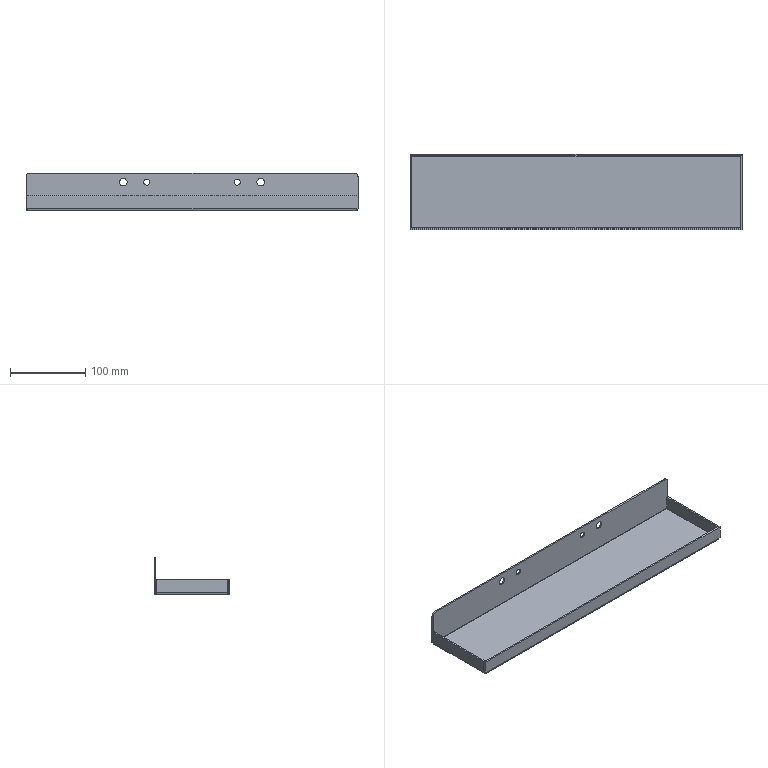Part | SolidWorks | features ICE 4, Extrusion 1, Fillet 1, FlatPattern 1, Rip 1, SheetMetal 1, Shell 1, SolidToSheetMetal 1 | 1 solid | 52 faces | box 440 x 100 x 50 mm | volume 150958 mm3 | plane 34 | cylinder 18 | commonest cylinder face diameters 10 x6 1 x4 5 x4 8 x4
STEP:
#1=CARTESIAN_POINT('',(-91.,50.,33.));
#2=VERTEX_POINT('',#1);
#3=CARTESIAN_POINT('',(-91.,50.,43.));
#4=VERTEX_POINT('',#3);
#5=CARTESIAN_POINT('',(-91.,50.,38.));
#6=DIRECTION('',(0.,1.,0.));
#7=DIRECTION('',(0.,0.,1.));
#8=AXIS2_PLACEMENT_3D('',#5,#6,#7);
#9=CIRCLE('',#8,5.);
#10=EDGE_CURVE('',#2,#4,#9,.T.);
#11=ORIENTED_EDGE('',*,*,#10,.T.);
#12=CARTESIAN_POINT('',(-91.,48.,43.));
#13=VERTEX_POINT('',#12);
#14=CARTESIAN_POINT('',(-91.,50.,43.));
#15=DIRECTION('',(0.,-1.,0.));
#16=VECTOR('',#15,1000.);
#17=LINE('',#14,#16);
#18=EDGE_CURVE('',#4,#13,#17,.T.);
#19=ORIENTED_EDGE('',*,*,#18,.T.);
#20=CARTESIAN_POINT('',(-91.,48.,33.));
#21=VERTEX_POINT('',#20);
#22=CARTESIAN_POINT('',(-91.,48.,38.));
#23=DIRECTION('',(0.,1.,0.));
#24=DIRECTION('',(0.,0.,1.));
#25=AXIS2_PLACEMENT_3D('',#22,#23,#24);
#26=CIRCLE('',#25,5.);
#27=EDGE_CURVE('',#21,#13,#26,.T.);
#28=ORIENTED_EDGE('',*,*,#27,.F.);
#29=CARTESIAN_POINT('',(-91.,50.,33.));
#30=DIRECTION('',(0.,-1.,0.));
#31=VECTOR('',#30,1000.);
#32=LINE('',#29,#31);
#33=EDGE_CURVE('',#2,#21,#32,.T.);
#34=ORIENTED_EDGE('',*,*,#33,.F.);
#35=EDGE_LOOP('',(#11,#19,#28,#34));
#36=FACE_OUTER_BOUND('',#35,.T.);
#37=CARTESIAN_POINT('',(-91.,50.,38.));
#38=DIRECTION('',(0.,-1.,0.));
#39=DIRECTION('',(0.,0.,-1.));
#40=AXIS2_PLACEMENT_3D('',#37,#38,#39);
#41=CYLINDRICAL_SURFACE('',#40,5.);
#42=ADVANCED_FACE('',(#36),#41,.F.);
#43=CARTESIAN_POINT('',(91.,50.,33.));
#44=VERTEX_POINT('',#43);
#45=CARTESIAN_POINT('',(91.,50.,43.));
#46=VERTEX_POINT('',#45);
#47=CARTESIAN_POINT('',(91.,50.,38.));
#48=DIRECTION('',(0.,1.,0.));
#49=DIRECTION('',(0.,0.,1.));
#50=AXIS2_PLACEMENT_3D('',#47,#48,#49);
#51=CIRCLE('',#50,5.);
#52=EDGE_CURVE('',#44,#46,#51,.T.);
#53=ORIENTED_EDGE('',*,*,#52,.T.);
#54=CARTESIAN_POINT('',(91.,48.,43.));
#55=VERTEX_POINT('',#54);
#56=CARTESIAN_POINT('',(91.,50.,43.));
#57=DIRECTION('',(0.,-1.,0.));
#58=VECTOR('',#57,1000.);
#59=LINE('',#56,#58);
#60=EDGE_CURVE('',#46,#55,#59,.T.);
#61=ORIENTED_EDGE('',*,*,#60,.T.);
#62=CARTESIAN_POINT('',(91.,48.,33.));
#63=VERTEX_POINT('',#62);
#64=CARTESIAN_POINT('',(91.,48.,38.));
#65=DIRECTION('',(0.,1.,0.));
#66=DIRECTION('',(0.,0.,1.));
#67=AXIS2_PLACEMENT_3D('',#64,#65,#66);
#68=CIRCLE('',#67,5.);
#69=EDGE_CURVE('',#63,#55,#68,.T.);
#70=ORIENTED_EDGE('',*,*,#69,.F.);
#71=CARTESIAN_POINT('',(91.,50.,33.));
#72=DIRECTION('',(0.,-1.,0.));
#73=VECTOR('',#72,1000.);
#74=LINE('',#71,#73);
#75=EDGE_CURVE('',#44,#63,#74,.T.);
#76=ORIENTED_EDGE('',*,*,#75,.F.);
#77=EDGE_LOOP('',(#53,#61,#70,#76));
#78=FACE_OUTER_BOUND('',#77,.T.);
#79=CARTESIAN_POINT('',(91.,50.,38.));
#80=DIRECTION('',(0.,-1.,0.));
#81=DIRECTION('',(0.,0.,-1.));
#82=AXIS2_PLACEMENT_3D('',#79,#80,#81);
#83=CYLINDRICAL_SURFACE('',#82,5.);
#84=ADVANCED_FACE('',(#78),#83,.F.);
#85=CARTESIAN_POINT('',(60.,50.,42.));
#86=VERTEX_POINT('',#85);
#87=CARTESIAN_POINT('',(60.,50.,34.));
#88=VERTEX_POINT('',#87);
#89=CARTESIAN_POINT('',(60.,50.,38.));
#90=DIRECTION('',(0.,-1.,0.));
#91=DIRECTION('',(0.,0.,-1.));
#92=AXIS2_PLACEMENT_3D('',#89,#90,#91);
#93=CIRCLE('',#92,4.);
#94=EDGE_CURVE('',#86,#88,#93,.T.);
#95=ORIENTED_EDGE('',*,*,#94,.F.);
#96=CARTESIAN_POINT('',(60.,48.,42.));
#97=VERTEX_POINT('',#96);
#98=CARTESIAN_POINT('',(60.,50.,42.));
#99=DIRECTION('',(0.,-1.,0.));
#100=VECTOR('',#99,1000.);
#101=LINE('',#98,#100);
#102=EDGE_CURVE('',#86,#97,#101,.T.);
#103=ORIENTED_EDGE('',*,*,#102,.T.);
#104=CARTESIAN_POINT('',(60.,48.,34.));
#105=VERTEX_POINT('',#104);
#106=CARTESIAN_POINT('',(60.,48.,38.));
#107=DIRECTION('',(0.,-1.,0.));
#108=DIRECTION('',(0.,0.,-1.));
#109=AXIS2_PLACEMENT_3D('',#106,#107,#108);
#110=CIRCLE('',#109,4.);
#111=EDGE_CURVE('',#97,#105,#110,.T.);
#112=ORIENTED_EDGE('',*,*,#111,.T.);
#113=CARTESIAN_POINT('',(60.,50.,34.));
#114=DIRECTION('',(0.,-1.,0.));
#115=VECTOR('',#114,1000.);
#116=LINE('',#113,#115);
#117=EDGE_CURVE('',#88,#105,#116,.T.);
#118=ORIENTED_EDGE('',*,*,#117,.F.);
#119=EDGE_LOOP('',(#95,#103,#112,#118));
#120=FACE_OUTER_BOUND('',#119,.T.);
#121=CARTESIAN_POINT('',(60.,50.,38.));
#122=DIRECTION('',(0.,-1.,0.));
#123=DIRECTION('',(0.,0.,-1.));
#124=AXIS2_PLACEMENT_3D('',#121,#122,#123);
#125=CYLINDRICAL_SURFACE('',#124,4.);
#126=ADVANCED_FACE('',(#120),#125,.F.);
#127=CARTESIAN_POINT('',(-60.,50.,42.));
#128=VERTEX_POINT('',#127);
#129=CARTESIAN_POINT('',(-60.,50.,34.));
#130=VERTEX_POINT('',#129);
#131=CARTESIAN_POINT('',(-60.,50.,38.));
#132=DIRECTION('',(0.,-1.,0.));
#133=DIRECTION('',(0.,0.,-1.));
#134=AXIS2_PLACEMENT_3D('',#131,#132,#133);
#135=CIRCLE('',#134,4.);
#136=EDGE_CURVE('',#128,#130,#135,.T.);
#137=ORIENTED_EDGE('',*,*,#136,.F.);
#138=CARTESIAN_POINT('',(-60.,48.,42.));
#139=VERTEX_POINT('',#138);
#140=CARTESIAN_POINT('',(-60.,50.,42.));
#141=DIRECTION('',(0.,-1.,0.));
#142=VECTOR('',#141,1000.);
#143=LINE('',#140,#142);
#144=EDGE_CURVE('',#128,#139,#143,.T.);
#145=ORIENTED_EDGE('',*,*,#144,.T.);
#146=CARTESIAN_POINT('',(-60.,48.,34.));
#147=VERTEX_POINT('',#146);
#148=CARTESIAN_POINT('',(-60.,48.,38.));
#149=DIRECTION('',(0.,-1.,0.));
#150=DIRECTION('',(0.,0.,-1.));
#151=AXIS2_PLACEMENT_3D('',#148,#149,#150);
#152=CIRCLE('',#151,4.);
#153=EDGE_CURVE('',#139,#147,#152,.T.);
#154=ORIENTED_EDGE('',*,*,#153,.T.);
#155=CARTESIAN_POINT('',(-60.,50.,34.));
#156=DIRECTION('',(0.,-1.,0.));
#157=VECTOR('',#156,1000.);
#158=LINE('',#155,#157);
#159=EDGE_CURVE('',#130,#147,#158,.T.);
#160=ORIENTED_EDGE('',*,*,#159,.F.);
#161=EDGE_LOOP('',(#137,#145,#154,#160));
#162=FACE_OUTER_BOUND('',#161,.T.);
#163=CARTESIAN_POINT('',(-60.,50.,38.));
#164=DIRECTION('',(0.,-1.,0.));
#165=DIRECTION('',(0.,0.,-1.));
#166=AXIS2_PLACEMENT_3D('',#163,#164,#165);
#167=CYLINDRICAL_SURFACE('',#166,4.);
#168=ADVANCED_FACE('',(#162),#167,.F.);
#169=CARTESIAN_POINT('',(-217.5,47.5,2.));
#170=VERTEX_POINT('',#169);
#171=CARTESIAN_POINT('',(-217.5,47.5,0.));
#172=VERTEX_POINT('',#171);
#173=CARTESIAN_POINT('',(-217.5,47.5,0.));
#174=DIRECTION('',(0.,0.,-1.));
#175=VECTOR('',#174,1000.);
#176=LINE('',#173,#175);
#177=EDGE_CURVE('',#170,#172,#176,.T.);
#178=ORIENTED_EDGE('',*,*,#177,.F.);
#179=CARTESIAN_POINT('',(-217.5,48.,2.5));
#180=VERTEX_POINT('',#179);
#181=CARTESIAN_POINT('',(-217.5,47.5,2.5));
#182=DIRECTION('',(1.,0.,0.));
#183=DIRECTION('',(0.,0.,1.));
#184=AXIS2_PLACEMENT_3D('',#181,#182,#183);
#185=CIRCLE('',#184,0.5);
#186=EDGE_CURVE('',#170,#180,#185,.T.);
#187=ORIENTED_EDGE('',*,*,#186,.T.);
#188=CARTESIAN_POINT('',(-217.5,50.,2.5));
#189=VERTEX_POINT('',#188);
#190=CARTESIAN_POINT('',(-217.5,50.,2.5));
#191=DIRECTION('',(0.,1.,0.));
#192=VECTOR('',#191,1000.);
#193=LINE('',#190,#192);
#194=EDGE_CURVE('',#180,#189,#193,.T.);
#195=ORIENTED_EDGE('',*,*,#194,.T.);
#196=CARTESIAN_POINT('',(-217.5,47.5,2.5));
#197=DIRECTION('',(1.,0.,0.));
#198=DIRECTION('',(0.,0.,1.));
#199=AXIS2_PLACEMENT_3D('',#196,#197,#198);
#200=CIRCLE('',#199,2.5);
#201=EDGE_CURVE('',#172,#189,#200,.T.);
#202=ORIENTED_EDGE('',*,*,#201,.F.);
#203=EDGE_LOOP('',(#178,#187,#195,#202));
#204=FACE_OUTER_BOUND('',#203,.T.);
#205=CARTESIAN_POINT('',(-217.5,47.5,2.5));
#206=DIRECTION('',(1.,0.,0.));
#207=DIRECTION('',(0.,0.,-1.));
#208=AXIS2_PLACEMENT_3D('',#205,#206,#207);
#209=PLANE('',#208);
#210=ADVANCED_FACE('',(#204),#209,.F.);
#211=ORIENTED_EDGE('',*,*,#194,.F.);
#212=CARTESIAN_POINT('',(-220.,48.,2.5));
#213=VERTEX_POINT('',#212);
#214=CARTESIAN_POINT('',(-220.,48.,2.5));
#215=DIRECTION('',(1.,0.,0.));
#216=VECTOR('',#215,1000.);
#217=LINE('',#214,#216);
#218=EDGE_CURVE('',#213,#180,#217,.T.);
#219=ORIENTED_EDGE('',*,*,#218,.F.);
#220=CARTESIAN_POINT('',(-220.,50.,2.5));
#221=VERTEX_POINT('',#220);
#222=CARTESIAN_POINT('',(-220.,50.,2.5));
#223=DIRECTION('',(0.,1.,0.));
#224=VECTOR('',#223,1000.);
#225=LINE('',#222,#224);
#226=EDGE_CURVE('',#213,#221,#225,.T.);
#227=ORIENTED_EDGE('',*,*,#226,.T.);
#228=CARTESIAN_POINT('',(-220.,50.,2.5));
#229=DIRECTION('',(1.,0.,0.));
#230=VECTOR('',#229,1000.);
#231=LINE('',#228,#230);
#232=EDGE_CURVE('',#221,#189,#231,.T.);
#233=ORIENTED_EDGE('',*,*,#232,.T.);
#234=EDGE_LOOP('',(#211,#219,#227,#233));
#235=FACE_OUTER_BOUND('',#234,.T.);
#236=CARTESIAN_POINT('',(-220.,50.,2.5));
#237=DIRECTION('',(0.,0.,-1.));
#238=DIRECTION('',(1.,0.,0.));
#239=AXIS2_PLACEMENT_3D('',#236,#237,#238);
#240=PLANE('',#239);
#241=ADVANCED_FACE('',(#235),#240,.T.);
#242=ORIENTED_EDGE('',*,*,#226,.F.);
#243=CARTESIAN_POINT('',(-220.,48.,45.));
#244=VERTEX_POINT('',#243);
#245=CARTESIAN_POINT('',(-220.,48.,20.));
#246=DIRECTION('',(0.,0.,-1.));
#247=VECTOR('',#246,1000.);
#248=LINE('',#245,#247);
#249=EDGE_CURVE('',#244,#213,#248,.T.);
#250=ORIENTED_EDGE('',*,*,#249,.F.);
#251=CARTESIAN_POINT('',(-220.,50.,45.));
#252=VERTEX_POINT('',#251);
#253=CARTESIAN_POINT('',(-220.,50.,45.));
#254=DIRECTION('',(0.,1.,0.));
#255=VECTOR('',#254,1000.);
#256=LINE('',#253,#255);
#257=EDGE_CURVE('',#244,#252,#256,.T.);
#258=ORIENTED_EDGE('',*,*,#257,.T.);
#259=CARTESIAN_POINT('',(-220.,50.,20.));
#260=DIRECTION('',(0.,0.,-1.));
#261=VECTOR('',#260,1000.);
#262=LINE('',#259,#261);
#263=EDGE_CURVE('',#252,#221,#262,.T.);
#264=ORIENTED_EDGE('',*,*,#263,.T.);
#265=EDGE_LOOP('',(#242,#250,#258,#264));
#266=FACE_OUTER_BOUND('',#265,.T.);
#267=CARTESIAN_POINT('',(-220.,50.,20.));
#268=DIRECTION('',(-1.,0.,0.));
#269=DIRECTION('',(0.,0.,-1.));
#270=AXIS2_PLACEMENT_3D('',#267,#268,#269);
#271=PLANE('',#270);
#272=ADVANCED_FACE('',(#266),#271,.T.);
#273=ORIENTED_EDGE('',*,*,#257,.F.);
#274=CARTESIAN_POINT('',(-215.,48.,50.));
#275=VERTEX_POINT('',#274);
#276=CARTESIAN_POINT('',(-215.,48.,45.));
#277=DIRECTION('',(0.,1.,0.));
#278=DIRECTION('',(0.,0.,-1.));
#279=AXIS2_PLACEMENT_3D('',#276,#277,#278);
#280=CIRCLE('',#279,5.);
#281=EDGE_CURVE('',#244,#275,#280,.T.);
#282=ORIENTED_EDGE('',*,*,#281,.T.);
#283=CARTESIAN_POINT('',(-215.,50.,50.));
#284=VERTEX_POINT('',#283);
#285=CARTESIAN_POINT('',(-215.,50.,50.));
#286=DIRECTION('',(0.,1.,0.));
#287=VECTOR('',#286,1000.);
#288=LINE('',#285,#287);
#289=EDGE_CURVE('',#275,#284,#288,.T.);
#290=ORIENTED_EDGE('',*,*,#289,.T.);
#291=CARTESIAN_POINT('',(-215.,50.,45.));
#292=DIRECTION('',(0.,1.,0.));
#293=DIRECTION('',(0.,0.,-1.));
#294=AXIS2_PLACEMENT_3D('',#291,#292,#293);
#295=CIRCLE('',#294,5.);
#296=EDGE_CURVE('',#252,#284,#295,.T.);
#297=ORIENTED_EDGE('',*,*,#296,.F.);
#298=EDGE_LOOP('',(#273,#282,#290,#297));
#299=FACE_OUTER_BOUND('',#298,.T.);
#300=CARTESIAN_POINT('',(-215.,50.,45.));
#301=DIRECTION('',(0.,-1.,0.));
#302=DIRECTION('',(0.,0.,-1.));
#303=AXIS2_PLACEMENT_3D('',#300,#301,#302);
#304=CYLINDRICAL_SURFACE('',#303,5.);
#305=ADVANCED_FACE('',(#299),#304,.T.);
#306=ORIENTED_EDGE('',*,*,#289,.F.);
#307=CARTESIAN_POINT('',(215.,48.,50.));
#308=VERTEX_POINT('',#307);
#309=CARTESIAN_POINT('',(-220.,48.,50.));
#310=DIRECTION('',(1.,0.,0.));
#311=VECTOR('',#310,1000.);
#312=LINE('',#309,#311);
#313=EDGE_CURVE('',#275,#308,#312,.T.);
#314=ORIENTED_EDGE('',*,*,#313,.T.);
#315=CARTESIAN_POINT('',(215.,50.,50.));
#316=VERTEX_POINT('',#315);
#317=CARTESIAN_POINT('',(215.,50.,50.));
#318=DIRECTION('',(0.,1.,0.));
#319=VECTOR('',#318,1000.);
#320=LINE('',#317,#319);
#321=EDGE_CURVE('',#308,#316,#320,.T.);
#322=ORIENTED_EDGE('',*,*,#321,.T.);
#323=CARTESIAN_POINT('',(220.,50.,50.));
#324=DIRECTION('',(1.,0.,0.));
#325=VECTOR('',#324,1000.);
#326=LINE('',#323,#325);
#327=EDGE_CURVE('',#284,#316,#326,.T.);
#328=ORIENTED_EDGE('',*,*,#327,.F.);
#329=EDGE_LOOP('',(#306,#314,#322,#328));
#330=FACE_OUTER_BOUND('',#329,.T.);
#331=CARTESIAN_POINT('',(220.,50.,50.));
#332=DIRECTION('',(0.,0.,-1.));
#333=DIRECTION('',(1.,0.,0.));
#334=AXIS2_PLACEMENT_3D('',#331,#332,#333);
#335=PLANE('',#334);
#336=ADVANCED_FACE('',(#330),#335,.F.);
#337=ORIENTED_EDGE('',*,*,#321,.F.);
#338=CARTESIAN_POINT('',(220.,48.,45.));
#339=VERTEX_POINT('',#338);
#340=CARTESIAN_POINT('',(215.,48.,45.));
#341=DIRECTION('',(0.,1.,0.));
#342=DIRECTION('',(0.,0.,-1.));
#343=AXIS2_PLACEMENT_3D('',#340,#341,#342);
#344=CIRCLE('',#343,5.);
#345=EDGE_CURVE('',#308,#339,#344,.T.);
#346=ORIENTED_EDGE('',*,*,#345,.T.);
#347=CARTESIAN_POINT('',(220.,50.,45.));
#348=VERTEX_POINT('',#347);
#349=CARTESIAN_POINT('',(220.,50.,45.));
#350=DIRECTION('',(0.,1.,0.));
#351=VECTOR('',#350,1000.);
#352=LINE('',#349,#351);
#353=EDGE_CURVE('',#339,#348,#352,.T.);
#354=ORIENTED_EDGE('',*,*,#353,.T.);
#355=CARTESIAN_POINT('',(215.,50.,45.));
#356=DIRECTION('',(0.,1.,0.));
#357=DIRECTION('',(0.,0.,-1.));
#358=AXIS2_PLACEMENT_3D('',#355,#356,#357);
#359=CIRCLE('',#358,5.);
#360=EDGE_CURVE('',#316,#348,#359,.T.);
#361=ORIENTED_EDGE('',*,*,#360,.F.);
#362=EDGE_LOOP('',(#337,#346,#354,#361));
#363=FACE_OUTER_BOUND('',#362,.T.);
#364=CARTESIAN_POINT('',(215.,50.,45.));
#365=DIRECTION('',(0.,-1.,0.));
#366=DIRECTION('',(0.,0.,-1.));
#367=AXIS2_PLACEMENT_3D('',#364,#365,#366);
#368=CYLINDRICAL_SURFACE('',#367,5.);
#369=ADVANCED_FACE('',(#363),#368,.T.);
#370=ORIENTED_EDGE('',*,*,#353,.F.);
#371=CARTESIAN_POINT('',(220.,48.,2.5));
#372=VERTEX_POINT('',#371);
#373=CARTESIAN_POINT('',(220.,48.,20.));
#374=DIRECTION('',(0.,0.,-1.));
#375=VECTOR('',#374,1000.);
#376=LINE('',#373,#375);
#377=EDGE_CURVE('',#339,#372,#376,.T.);
#378=ORIENTED_EDGE('',*,*,#377,.T.);
#379=CARTESIAN_POINT('',(220.,50.,2.5));
#380=VERTEX_POINT('',#379);
#381=CARTESIAN_POINT('',(220.,50.,2.5));
#382=DIRECTION('',(0.,1.,0.));
#383=VECTOR('',#382,1000.);
#384=LINE('',#381,#383);
#385=EDGE_CURVE('',#372,#380,#384,.T.);
#386=ORIENTED_EDGE('',*,*,#385,.T.);
#387=CARTESIAN_POINT('',(220.,50.,20.));
#388=DIRECTION('',(0.,0.,-1.));
#389=VECTOR('',#388,1000.);
#390=LINE('',#387,#389);
#391=EDGE_CURVE('',#348,#380,#390,.T.);
#392=ORIENTED_EDGE('',*,*,#391,.F.);
#393=EDGE_LOOP('',(#370,#378,#386,#392));
#394=FACE_OUTER_BOUND('',#393,.T.);
#395=CARTESIAN_POINT('',(220.,50.,20.));
#396=DIRECTION('',(-1.,0.,0.));
#397=DIRECTION('',(0.,0.,-1.));
#398=AXIS2_PLACEMENT_3D('',#395,#396,#397);
#399=PLANE('',#398);
#400=ADVANCED_FACE('',(#394),#399,.F.);
#401=ORIENTED_EDGE('',*,*,#385,.F.);
#402=CARTESIAN_POINT('',(217.5,48.,2.5));
#403=VERTEX_POINT('',#402);
#404=CARTESIAN_POINT('',(-220.,48.,2.5));
#405=DIRECTION('',(1.,0.,0.));
#406=VECTOR('',#405,1000.);
#407=LINE('',#404,#406);
#408=EDGE_CURVE('',#403,#372,#407,.T.);
#409=ORIENTED_EDGE('',*,*,#408,.F.);
#410=CARTESIAN_POINT('',(217.5,50.,2.5));
#411=VERTEX_POINT('',#410);
#412=CARTESIAN_POINT('',(217.5,50.,2.5));
#413=DIRECTION('',(0.,1.,0.));
#414=VECTOR('',#413,1000.);
#415=LINE('',#412,#414);
#416=EDGE_CURVE('',#403,#411,#415,.T.);
#417=ORIENTED_EDGE('',*,*,#416,.T.);
#418=CARTESIAN_POINT('',(220.,50.,2.5));
#419=DIRECTION('',(1.,0.,0.));
#420=VECTOR('',#419,1000.);
#421=LINE('',#418,#420);
#422=EDGE_CURVE('',#411,#380,#421,.T.);
#423=ORIENTED_EDGE('',*,*,#422,.T.);
#424=EDGE_LOOP('',(#401,#409,#417,#423));
#425=FACE_OUTER_BOUND('',#424,.T.);
#426=CARTESIAN_POINT('',(220.,50.,2.5));
#427=DIRECTION('',(0.,0.,-1.));
#428=DIRECTION('',(1.,0.,0.));
#429=AXIS2_PLACEMENT_3D('',#426,#427,#428);
#430=PLANE('',#429);
#431=ADVANCED_FACE('',(#425),#430,.T.);
#432=ORIENTED_EDGE('',*,*,#416,.F.);
#433=CARTESIAN_POINT('',(217.5,47.5,2.));
#434=VERTEX_POINT('',#433);
#435=CARTESIAN_POINT('',(217.5,47.5,2.5));
#436=DIRECTION('',(-1.,0.,0.));
#437=DIRECTION('',(0.,0.,1.));
#438=AXIS2_PLACEMENT_3D('',#435,#436,#437);
#439=CIRCLE('',#438,0.5);
#440=EDGE_CURVE('',#403,#434,#439,.T.);
#441=ORIENTED_EDGE('',*,*,#440,.T.);
#442=CARTESIAN_POINT('',(217.5,47.5,0.));
#443=VERTEX_POINT('',#442);
#444=CARTESIAN_POINT('',(217.5,47.5,0.));
#445=DIRECTION('',(0.,0.,-1.));
#446=VECTOR('',#445,1000.);
#447=LINE('',#444,#446);
#448=EDGE_CURVE('',#434,#443,#447,.T.);
#449=ORIENTED_EDGE('',*,*,#448,.T.);
#450=CARTESIAN_POINT('',(217.5,47.5,2.5));
#451=DIRECTION('',(-1.,0.,0.));
#452=DIRECTION('',(0.,0.,1.));
#453=AXIS2_PLACEMENT_3D('',#450,#451,#452);
#454=CIRCLE('',#453,2.5);
#455=EDGE_CURVE('',#411,#443,#454,.T.);
#456=ORIENTED_EDGE('',*,*,#455,.F.);
#457=EDGE_LOOP('',(#432,#441,#449,#456));
#458=FACE_OUTER_BOUND('',#457,.T.);
#459=CARTESIAN_POINT('',(217.5,47.5,2.5));
#460=DIRECTION('',(1.,0.,0.));
#461=DIRECTION('',(0.,0.,-1.));
#462=AXIS2_PLACEMENT_3D('',#459,#460,#461);
#463=PLANE('',#462);
#464=ADVANCED_FACE('',(#458),#463,.T.);
#465=ORIENTED_EDGE('',*,*,#448,.F.);
#466=CARTESIAN_POINT('',(218.,47.5,2.5));
#467=VERTEX_POINT('',#466);
#468=CARTESIAN_POINT('',(217.5,47.5,2.5));
#469=DIRECTION('',(0.,-1.,0.));
#470=DIRECTION('',(-1.,0.,0.));
#471=AXIS2_PLACEMENT_3D('',#468,#469,#470);
#472=CIRCLE('',#471,0.5);
#473=EDGE_CURVE('',#434,#467,#472,.T.);
#474=ORIENTED_EDGE('',*,*,#473,.T.);
#475=CARTESIAN_POINT('',(220.,47.5,2.5));
#476=VERTEX_POINT('',#475);
#477=CARTESIAN_POINT('',(220.,47.5,2.5));
#478=DIRECTION('',(1.,0.,0.));
#479=VECTOR('',#478,1000.);
#480=LINE('',#477,#479);
#481=EDGE_CURVE('',#467,#476,#480,.T.);
#482=ORIENTED_EDGE('',*,*,#481,.T.);
#483=CARTESIAN_POINT('',(217.5,47.5,2.5));
#484=DIRECTION('',(0.,-1.,0.));
#485=DIRECTION('',(0.,0.,-1.));
#486=AXIS2_PLACEMENT_3D('',#483,#484,#485);
#487=CIRCLE('',#486,2.5);
#488=EDGE_CURVE('',#443,#476,#487,.T.);
#489=ORIENTED_EDGE('',*,*,#488,.F.);
#490=EDGE_LOOP('',(#465,#474,#482,#489));
#491=FACE_OUTER_BOUND('',#490,.T.);
#492=CARTESIAN_POINT('',(217.5,47.5,2.5));
#493=DIRECTION('',(0.,1.,0.));
#494=DIRECTION('',(0.,0.,1.));
#495=AXIS2_PLACEMENT_3D('',#492,#493,#494);
#496=PLANE('',#495);
#497=ADVANCED_FACE('',(#491),#496,.T.);
#498=ORIENTED_EDGE('',*,*,#481,.F.);
#499=CARTESIAN_POINT('',(218.,47.5,20.));
#500=VERTEX_POINT('',#499);
#501=CARTESIAN_POINT('',(218.,47.5,20.));
#502=DIRECTION('',(0.,0.,1.));
#503=VECTOR('',#502,1000.);
#504=LINE('',#501,#503);
#505=EDGE_CURVE('',#467,#500,#504,.T.);
#506=ORIENTED_EDGE('',*,*,#505,.T.);
#507=CARTESIAN_POINT('',(220.,47.5,20.));
#508=VERTEX_POINT('',#507);
#509=CARTESIAN_POINT('',(220.,47.5,20.));
#510=DIRECTION('',(1.,0.,0.));
#511=VECTOR('',#510,1000.);
#512=LINE('',#509,#511);
#513=EDGE_CURVE('',#500,#508,#512,.T.);
#514=ORIENTED_EDGE('',*,*,#513,.T.);
#515=CARTESIAN_POINT('',(220.,47.5,-11.));
#516=DIRECTION('',(0.,0.,1.));
#517=VECTOR('',#516,1000.);
#518=LINE('',#515,#517);
#519=EDGE_CURVE('',#476,#508,#518,.T.);
#520=ORIENTED_EDGE('',*,*,#519,.F.);
#521=EDGE_LOOP('',(#498,#506,#514,#520));
#522=FACE_OUTER_BOUND('',#521,.T.);
#523=CARTESIAN_POINT('',(220.,47.5,-11.));
#524=DIRECTION('',(0.,-1.,0.));
#525=DIRECTION('',(0.,0.,1.));
#526=AXIS2_PLACEMENT_3D('',#523,#524,#525);
#527=PLANE('',#526);
#528=ADVANCED_FACE('',(#522),#527,.F.);
#529=ORIENTED_EDGE('',*,*,#513,.F.);
#530=CARTESIAN_POINT('',(218.,-47.5,20.));
#531=VERTEX_POINT('',#530);
#532=CARTESIAN_POINT('',(218.,50.,20.));
#533=DIRECTION('',(0.,1.,0.));
#534=VECTOR('',#533,1000.);
#535=LINE('',#532,#534);
#536=EDGE_CURVE('',#531,#500,#535,.T.);
#537=ORIENTED_EDGE('',*,*,#536,.F.);
#538=CARTESIAN_POINT('',(220.,-47.5,20.));
#539=VERTEX_POINT('',#538);
#540=CARTESIAN_POINT('',(220.,-47.5,20.));
#541=DIRECTION('',(1.,0.,0.));
#542=VECTOR('',#541,1000.);
#543=LINE('',#540,#542);
#544=EDGE_CURVE('',#531,#539,#543,.T.);
#545=ORIENTED_EDGE('',*,*,#544,.T.);
#546=CARTESIAN_POINT('',(220.,50.,20.));
#547=DIRECTION('',(0.,1.,0.));
#548=VECTOR('',#547,1000.);
#549=LINE('',#546,#548);
#550=EDGE_CURVE('',#539,#508,#549,.T.);
#551=ORIENTED_EDGE('',*,*,#550,.T.);
#552=EDGE_LOOP('',(#529,#537,#545,#551));
#553=FACE_OUTER_BOUND('',#552,.T.);
#554=CARTESIAN_POINT('',(220.,50.,20.));
#555=DIRECTION('',(0.,0.,1.));
#556=DIRECTION('',(0.,1.,0.));
#557=AXIS2_PLACEMENT_3D('',#554,#555,#556);
#558=PLANE('',#557);
#559=ADVANCED_FACE('',(#553),#558,.T.);
#560=ORIENTED_EDGE('',*,*,#544,.F.);
#561=CARTESIAN_POINT('',(218.,-47.5,2.5));
#562=VERTEX_POINT('',#561);
#563=CARTESIAN_POINT('',(218.,-47.5,20.));
#564=DIRECTION('',(0.,0.,-1.));
#565=VECTOR('',#564,1000.);
#566=LINE('',#563,#565);
#567=EDGE_CURVE('',#531,#562,#566,.T.);
#568=ORIENTED_EDGE('',*,*,#567,.T.);
#569=CARTESIAN_POINT('',(220.,-47.5,2.5));
#570=VERTEX_POINT('',#569);
#571=CARTESIAN_POINT('',(220.,-47.5,2.5));
#572=DIRECTION('',(1.,0.,0.));
#573=VECTOR('',#572,1000.);
#574=LINE('',#571,#573);
#575=EDGE_CURVE('',#562,#570,#574,.T.);
#576=ORIENTED_EDGE('',*,*,#575,.T.);
#577=CARTESIAN_POINT('',(220.,-47.5,33.));
#578=DIRECTION('',(0.,0.,-1.));
#579=VECTOR('',#578,1000.);
#580=LINE('',#577,#579);
#581=EDGE_CURVE('',#539,#570,#580,.T.);
#582=ORIENTED_EDGE('',*,*,#581,.F.);
#583=EDGE_LOOP('',(#560,#568,#576,#582));
#584=FACE_OUTER_BOUND('',#583,.T.);
#585=CARTESIAN_POINT('',(220.,-47.5,33.));
#586=DIRECTION('',(0.,1.,0.));
#587=DIRECTION('',(0.,0.,-1.));
#588=AXIS2_PLACEMENT_3D('',#585,#586,#587);
#589=PLANE('',#588);
#590=ADVANCED_FACE('',(#584),#589,.F.);
#591=ORIENTED_EDGE('',*,*,#575,.F.);
#592=CARTESIAN_POINT('',(217.5,-47.5,2.));
#593=VERTEX_POINT('',#592);
#594=CARTESIAN_POINT('',(217.5,-47.5,2.5));
#595=DIRECTION('',(0.,1.,0.));
#596=DIRECTION('',(-1.,0.,0.));
#597=AXIS2_PLACEMENT_3D('',#594,#595,#596);
#598=CIRCLE('',#597,0.5);
#599=EDGE_CURVE('',#562,#593,#598,.T.);
#600=ORIENTED_EDGE('',*,*,#599,.T.);
#601=CARTESIAN_POINT('',(217.5,-47.5,0.));
#602=VERTEX_POINT('',#601);
#603=CARTESIAN_POINT('',(217.5,-47.5,0.));
#604=DIRECTION('',(0.,0.,-1.));
#605=VECTOR('',#604,1000.);
#606=LINE('',#603,#605);
#607=EDGE_CURVE('',#593,#602,#606,.T.);
#608=ORIENTED_EDGE('',*,*,#607,.T.);
#609=CARTESIAN_POINT('',(217.5,-47.5,2.5));
#610=DIRECTION('',(0.,1.,0.));
#611=DIRECTION('',(0.,0.,1.));
#612=AXIS2_PLACEMENT_3D('',#609,#610,#611);
#613=CIRCLE('',#612,2.5);
#614=EDGE_CURVE('',#570,#602,#613,.T.);
#615=ORIENTED_EDGE('',*,*,#614,.F.);
#616=EDGE_LOOP('',(#591,#600,#608,#615));
#617=FACE_OUTER_BOUND('',#616,.T.);
#618=CARTESIAN_POINT('',(217.5,-47.5,2.5));
#619=DIRECTION('',(0.,-1.,0.));
#620=DIRECTION('',(0.,0.,-1.));
#621=AXIS2_PLACEMENT_3D('',#618,#619,#620);
#622=PLANE('',#621);
#623=ADVANCED_FACE('',(#617),#622,.T.);
#624=ORIENTED_EDGE('',*,*,#607,.F.);
#625=CARTESIAN_POINT('',(217.5,-48.,2.5));
#626=VERTEX_POINT('',#625);
#627=CARTESIAN_POINT('',(217.5,-47.5,2.5));
#628=DIRECTION('',(-1.,0.,0.));
#629=DIRECTION('',(0.,0.,-1.));
#630=AXIS2_PLACEMENT_3D('',#627,#628,#629);
#631=CIRCLE('',#630,0.5);
#632=EDGE_CURVE('',#593,#626,#631,.T.);
#633=ORIENTED_EDGE('',*,*,#632,.T.);
#634=CARTESIAN_POINT('',(217.5,-50.,2.5));
#635=VERTEX_POINT('',#634);
#636=CARTESIAN_POINT('',(217.5,-50.,2.5));
#637=DIRECTION('',(0.,-1.,0.));
#638=VECTOR('',#637,1000.);
#639=LINE('',#636,#638);
#640=EDGE_CURVE('',#626,#635,#639,.T.);
#641=ORIENTED_EDGE('',*,*,#640,.T.);
#642=CARTESIAN_POINT('',(217.5,-47.5,2.5));
#643=DIRECTION('',(-1.,0.,0.));
#644=DIRECTION('',(0.,0.,-1.));
#645=AXIS2_PLACEMENT_3D('',#642,#643,#644);
#646=CIRCLE('',#645,2.5);
#647=EDGE_CURVE('',#602,#635,#646,.T.);
#648=ORIENTED_EDGE('',*,*,#647,.F.);
#649=EDGE_LOOP('',(#624,#633,#641,#648));
#650=FACE_OUTER_BOUND('',#649,.T.);
#651=CARTESIAN_POINT('',(217.5,-47.5,2.5));
#652=DIRECTION('',(-1.,0.,0.));
#653=DIRECTION('',(0.,0.,1.));
#654=AXIS2_PLACEMENT_3D('',#651,#652,#653);
#655=PLANE('',#654);
#656=ADVANCED_FACE('',(#650),#655,.F.);
#657=ORIENTED_EDGE('',*,*,#640,.F.);
#658=CARTESIAN_POINT('',(220.,-48.,2.5));
#659=VERTEX_POINT('',#658);
#660=CARTESIAN_POINT('',(-220.,-48.,2.5));
#661=DIRECTION('',(-1.,0.,0.));
#662=VECTOR('',#661,1000.);
#663=LINE('',#660,#662);
#664=EDGE_CURVE('',#659,#626,#663,.T.);
#665=ORIENTED_EDGE('',*,*,#664,.F.);
#666=CARTESIAN_POINT('',(220.,-50.,2.5));
#667=VERTEX_POINT('',#666);
#668=CARTESIAN_POINT('',(220.,-50.,2.5));
#669=DIRECTION('',(0.,-1.,0.));
#670=VECTOR('',#669,1000.);
#671=LINE('',#668,#670);
#672=EDGE_CURVE('',#659,#667,#671,.T.);
#673=ORIENTED_EDGE('',*,*,#672,.T.);
#674=CARTESIAN_POINT('',(220.,-50.,2.5));
#675=DIRECTION('',(-1.,0.,0.));
#676=VECTOR('',#675,1000.);
#677=LINE('',#674,#676);
#678=EDGE_CURVE('',#667,#635,#677,.T.);
#679=ORIENTED_EDGE('',*,*,#678,.T.);
#680=EDGE_LOOP('',(#657,#665,#673,#679));
#681=FACE_OUTER_BOUND('',#680,.T.);
#682=CARTESIAN_POINT('',(220.,-50.,2.5));
#683=DIRECTION('',(0.,0.,-1.));
#684=DIRECTION('',(-1.,0.,0.));
#685=AXIS2_PLACEMENT_3D('',#682,#683,#684);
#686=PLANE('',#685);
#687=ADVANCED_FACE('',(#681),#686,.T.);
#688=ORIENTED_EDGE('',*,*,#672,.F.);
#689=CARTESIAN_POINT('',(220.,-48.,20.));
#690=VERTEX_POINT('',#689);
#691=CARTESIAN_POINT('',(220.,-48.,20.));
#692=DIRECTION('',(0.,0.,-1.));
#693=VECTOR('',#692,1000.);
#694=LINE('',#691,#693);
#695=EDGE_CURVE('',#690,#659,#694,.T.);
#696=ORIENTED_EDGE('',*,*,#695,.F.);
#697=CARTESIAN_POINT('',(220.,-50.,20.));
#698=VERTEX_POINT('',#697);
#699=CARTESIAN_POINT('',(220.,-50.,20.));
#700=DIRECTION('',(0.,-1.,0.));
#701=VECTOR('',#700,1000.);
#702=LINE('',#699,#701);
#703=EDGE_CURVE('',#690,#698,#702,.T.);
#704=ORIENTED_EDGE('',*,*,#703,.T.);
#705=CARTESIAN_POINT('',(220.,-50.,20.));
#706=DIRECTION('',(0.,0.,-1.));
#707=VECTOR('',#706,1000.);
#708=LINE('',#705,#707);
#709=EDGE_CURVE('',#698,#667,#708,.T.);
#710=ORIENTED_EDGE('',*,*,#709,.T.);
#711=EDGE_LOOP('',(#688,#696,#704,#710));
#712=FACE_OUTER_BOUND('',#711,.T.);
#713=CARTESIAN_POINT('',(220.,-50.,20.));
#714=DIRECTION('',(1.,0.,0.));
#715=DIRECTION('',(0.,0.,-1.));
#716=AXIS2_PLACEMENT_3D('',#713,#714,#715);
#717=PLANE('',#716);
#718=ADVANCED_FACE('',(#712),#717,.T.);
#719=ORIENTED_EDGE('',*,*,#703,.F.);
#720=CARTESIAN_POINT('',(-220.,-48.,20.));
#721=VERTEX_POINT('',#720);
#722=CARTESIAN_POINT('',(-220.,-48.,20.));
#723=DIRECTION('',(1.,0.,0.));
#724=VECTOR('',#723,1000.);
#725=LINE('',#722,#724);
#726=EDGE_CURVE('',#721,#690,#725,.T.);
#727=ORIENTED_EDGE('',*,*,#726,.F.);
#728=CARTESIAN_POINT('',(-220.,-50.,20.));
#729=VERTEX_POINT('',#728);
#730=CARTESIAN_POINT('',(-220.,-50.,20.));
#731=DIRECTION('',(0.,-1.,0.));
#732=VECTOR('',#731,1000.);
#733=LINE('',#730,#732);
#734=EDGE_CURVE('',#721,#729,#733,.T.);
#735=ORIENTED_EDGE('',*,*,#734,.T.);
#736=CARTESIAN_POINT('',(-220.,-50.,20.));
#737=DIRECTION('',(1.,0.,0.));
#738=VECTOR('',#737,1000.);
#739=LINE('',#736,#738);
#740=EDGE_CURVE('',#729,#698,#739,.T.);
#741=ORIENTED_EDGE('',*,*,#740,.T.);
#742=EDGE_LOOP('',(#719,#727,#735,#741));
#743=FACE_OUTER_BOUND('',#742,.T.);
#744=CARTESIAN_POINT('',(-220.,-50.,20.));
#745=DIRECTION('',(0.,0.,1.));
#746=DIRECTION('',(1.,0.,0.));
#747=AXIS2_PLACEMENT_3D('',#744,#745,#746);
#748=PLANE('',#747);
#749=ADVANCED_FACE('',(#743),#748,.T.);
#750=ORIENTED_EDGE('',*,*,#734,.F.);
#751=CARTESIAN_POINT('',(-220.,-48.,2.5));
#752=VERTEX_POINT('',#751);
#753=CARTESIAN_POINT('',(-220.,-48.,20.));
#754=DIRECTION('',(0.,0.,-1.));
#755=VECTOR('',#754,1000.);
#756=LINE('',#753,#755);
#757=EDGE_CURVE('',#721,#752,#756,.T.);
#758=ORIENTED_EDGE('',*,*,#757,.T.);
#759=CARTESIAN_POINT('',(-220.,-50.,2.5));
#760=VERTEX_POINT('',#759);
#761=CARTESIAN_POINT('',(-220.,-50.,2.5));
#762=DIRECTION('',(0.,-1.,0.));
#763=VECTOR('',#762,1000.);
#764=LINE('',#761,#763);
#765=EDGE_CURVE('',#752,#760,#764,.T.);
#766=ORIENTED_EDGE('',*,*,#765,.T.);
#767=CARTESIAN_POINT('',(-220.,-50.,20.));
#768=DIRECTION('',(0.,0.,-1.));
#769=VECTOR('',#768,1000.);
#770=LINE('',#767,#769);
#771=EDGE_CURVE('',#729,#760,#770,.T.);
#772=ORIENTED_EDGE('',*,*,#771,.F.);
#773=EDGE_LOOP('',(#750,#758,#766,#772));
#774=FACE_OUTER_BOUND('',#773,.T.);
#775=CARTESIAN_POINT('',(-220.,-50.,20.));
#776=DIRECTION('',(1.,0.,0.));
#777=DIRECTION('',(0.,0.,-1.));
#778=AXIS2_PLACEMENT_3D('',#775,#776,#777);
#779=PLANE('',#778);
#780=ADVANCED_FACE('',(#774),#779,.F.);
#781=ORIENTED_EDGE('',*,*,#765,.F.);
#782=CARTESIAN_POINT('',(-217.5,-48.,2.5));
#783=VERTEX_POINT('',#782);
#784=CARTESIAN_POINT('',(-220.,-48.,2.5));
#785=DIRECTION('',(-1.,0.,0.));
#786=VECTOR('',#785,1000.);
#787=LINE('',#784,#786);
#788=EDGE_CURVE('',#783,#752,#787,.T.);
#789=ORIENTED_EDGE('',*,*,#788,.F.);
#790=CARTESIAN_POINT('',(-217.5,-50.,2.5));
#791=VERTEX_POINT('',#790);
#792=CARTESIAN_POINT('',(-217.5,-50.,2.5));
#793=DIRECTION('',(0.,-1.,0.));
#794=VECTOR('',#793,1000.);
#795=LINE('',#792,#794);
#796=EDGE_CURVE('',#783,#791,#795,.T.);
#797=ORIENTED_EDGE('',*,*,#796,.T.);
#798=CARTESIAN_POINT('',(-220.,-50.,2.5));
#799=DIRECTION('',(-1.,0.,0.));
#800=VECTOR('',#799,1000.);
#801=LINE('',#798,#800);
#802=EDGE_CURVE('',#791,#760,#801,.T.);
#803=ORIENTED_EDGE('',*,*,#802,.T.);
#804=EDGE_LOOP('',(#781,#789,#797,#803));
#805=FACE_OUTER_BOUND('',#804,.T.);
#806=CARTESIAN_POINT('',(-220.,-50.,2.5));
#807=DIRECTION('',(0.,0.,-1.));
#808=DIRECTION('',(-1.,0.,0.));
#809=AXIS2_PLACEMENT_3D('',#806,#807,#808);
#810=PLANE('',#809);
#811=ADVANCED_FACE('',(#805),#810,.T.);
#812=ORIENTED_EDGE('',*,*,#796,.F.);
#813=CARTESIAN_POINT('',(-217.5,-47.5,2.));
#814=VERTEX_POINT('',#813);
#815=CARTESIAN_POINT('',(-217.5,-47.5,2.5));
#816=DIRECTION('',(1.,0.,0.));
#817=DIRECTION('',(0.,0.,-1.));
#818=AXIS2_PLACEMENT_3D('',#815,#816,#817);
#819=CIRCLE('',#818,0.5);
#820=EDGE_CURVE('',#783,#814,#819,.T.);
#821=ORIENTED_EDGE('',*,*,#820,.T.);
#822=CARTESIAN_POINT('',(-217.5,-47.5,0.));
#823=VERTEX_POINT('',#822);
#824=CARTESIAN_POINT('',(-217.5,-47.5,0.));
#825=DIRECTION('',(0.,0.,-1.));
#826=VECTOR('',#825,1000.);
#827=LINE('',#824,#826);
#828=EDGE_CURVE('',#814,#823,#827,.T.);
#829=ORIENTED_EDGE('',*,*,#828,.T.);
#830=CARTESIAN_POINT('',(-217.5,-47.5,2.5));
#831=DIRECTION('',(1.,0.,0.));
#832=DIRECTION('',(0.,0.,-1.));
#833=AXIS2_PLACEMENT_3D('',#830,#831,#832);
#834=CIRCLE('',#833,2.5);
#835=EDGE_CURVE('',#791,#823,#834,.T.);
#836=ORIENTED_EDGE('',*,*,#835,.F.);
#837=EDGE_LOOP('',(#812,#821,#829,#836));
#838=FACE_OUTER_BOUND('',#837,.T.);
#839=CARTESIAN_POINT('',(-217.5,-47.5,2.5));
#840=DIRECTION('',(-1.,0.,0.));
#841=DIRECTION('',(0.,0.,1.));
#842=AXIS2_PLACEMENT_3D('',#839,#840,#841);
#843=PLANE('',#842);
#844=ADVANCED_FACE('',(#838),#843,.T.);
#845=ORIENTED_EDGE('',*,*,#828,.F.);
#846=CARTESIAN_POINT('',(-218.,-47.5,2.5));
#847=VERTEX_POINT('',#846);
#848=CARTESIAN_POINT('',(-217.5,-47.5,2.5));
#849=DIRECTION('',(0.,1.,0.));
#850=DIRECTION('',(0.,0.,-1.));
#851=AXIS2_PLACEMENT_3D('',#848,#849,#850);
#852=CIRCLE('',#851,0.5);
#853=EDGE_CURVE('',#814,#847,#852,.T.);
#854=ORIENTED_EDGE('',*,*,#853,.T.);
#855=CARTESIAN_POINT('',(-220.,-47.5,2.5));
#856=VERTEX_POINT('',#855);
#857=CARTESIAN_POINT('',(-220.,-47.5,2.5));
#858=DIRECTION('',(-1.,0.,0.));
#859=VECTOR('',#858,1000.);
#860=LINE('',#857,#859);
#861=EDGE_CURVE('',#847,#856,#860,.T.);
#862=ORIENTED_EDGE('',*,*,#861,.T.);
#863=CARTESIAN_POINT('',(-217.5,-47.5,2.5));
#864=DIRECTION('',(0.,1.,0.));
#865=DIRECTION('',(0.,0.,1.));
#866=AXIS2_PLACEMENT_3D('',#863,#864,#865);
#867=CIRCLE('',#866,2.5);
#868=EDGE_CURVE('',#823,#856,#867,.T.);
#869=ORIENTED_EDGE('',*,*,#868,.F.);
#870=EDGE_LOOP('',(#845,#854,#862,#869));
#871=FACE_OUTER_BOUND('',#870,.T.);
#872=CARTESIAN_POINT('',(-217.5,-47.5,2.5));
#873=DIRECTION('',(0.,-1.,0.));
#874=DIRECTION('',(0.,0.,-1.));
#875=AXIS2_PLACEMENT_3D('',#872,#873,#874);
#876=PLANE('',#875);
#877=ADVANCED_FACE('',(#871),#876,.T.);
#878=ORIENTED_EDGE('',*,*,#861,.F.);
#879=CARTESIAN_POINT('',(-218.,-47.5,20.));
#880=VERTEX_POINT('',#879);
#881=CARTESIAN_POINT('',(-218.,-47.5,20.));
#882=DIRECTION('',(0.,0.,1.));
#883=VECTOR('',#882,1000.);
#884=LINE('',#881,#883);
#885=EDGE_CURVE('',#847,#880,#884,.T.);
#886=ORIENTED_EDGE('',*,*,#885,.T.);
#887=CARTESIAN_POINT('',(-220.,-47.5,20.));
#888=VERTEX_POINT('',#887);
#889=CARTESIAN_POINT('',(-220.,-47.5,20.));
#890=DIRECTION('',(-1.,0.,0.));
#891=VECTOR('',#890,1000.);
#892=LINE('',#889,#891);
#893=EDGE_CURVE('',#880,#888,#892,.T.);
#894=ORIENTED_EDGE('',*,*,#893,.T.);
#895=CARTESIAN_POINT('',(-220.,-47.5,-11.));
#896=DIRECTION('',(0.,0.,1.));
#897=VECTOR('',#896,1000.);
#898=LINE('',#895,#897);
#899=EDGE_CURVE('',#856,#888,#898,.T.);
#900=ORIENTED_EDGE('',*,*,#899,.F.);
#901=EDGE_LOOP('',(#878,#886,#894,#900));
#902=FACE_OUTER_BOUND('',#901,.T.);
#903=CARTESIAN_POINT('',(-220.,-47.5,-11.));
#904=DIRECTION('',(0.,1.,0.));
#905=DIRECTION('',(0.,0.,1.));
#906=AXIS2_PLACEMENT_3D('',#903,#904,#905);
#907=PLANE('',#906);
#908=ADVANCED_FACE('',(#902),#907,.F.);
#909=ORIENTED_EDGE('',*,*,#893,.F.);
#910=CARTESIAN_POINT('',(-218.,47.5,20.));
#911=VERTEX_POINT('',#910);
#912=CARTESIAN_POINT('',(-218.,50.,20.));
#913=DIRECTION('',(0.,-1.,0.));
#914=VECTOR('',#913,1000.);
#915=LINE('',#912,#914);
#916=EDGE_CURVE('',#911,#880,#915,.T.);
#917=ORIENTED_EDGE('',*,*,#916,.F.);
#918=CARTESIAN_POINT('',(-220.,47.5,20.));
#919=VERTEX_POINT('',#918);
#920=CARTESIAN_POINT('',(-220.,47.5,20.));
#921=DIRECTION('',(-1.,0.,0.));
#922=VECTOR('',#921,1000.);
#923=LINE('',#920,#922);
#924=EDGE_CURVE('',#911,#919,#923,.T.);
#925=ORIENTED_EDGE('',*,*,#924,.T.);
#926=CARTESIAN_POINT('',(-220.,50.,20.));
#927=DIRECTION('',(0.,-1.,0.));
#928=VECTOR('',#927,1000.);
#929=LINE('',#926,#928);
#930=EDGE_CURVE('',#919,#888,#929,.T.);
#931=ORIENTED_EDGE('',*,*,#930,.T.);
#932=EDGE_LOOP('',(#909,#917,#925,#931));
#933=FACE_OUTER_BOUND('',#932,.T.);
#934=CARTESIAN_POINT('',(-220.,50.,20.));
#935=DIRECTION('',(0.,0.,1.));
#936=DIRECTION('',(0.,-1.,0.));
#937=AXIS2_PLACEMENT_3D('',#934,#935,#936);
#938=PLANE('',#937);
#939=ADVANCED_FACE('',(#933),#938,.T.);
#940=ORIENTED_EDGE('',*,*,#924,.F.);
#941=CARTESIAN_POINT('',(-218.,47.5,2.5));
#942=VERTEX_POINT('',#941);
#943=CARTESIAN_POINT('',(-218.,47.5,20.));
#944=DIRECTION('',(0.,0.,-1.));
#945=VECTOR('',#944,1000.);
#946=LINE('',#943,#945);
#947=EDGE_CURVE('',#911,#942,#946,.T.);
#948=ORIENTED_EDGE('',*,*,#947,.T.);
#949=CARTESIAN_POINT('',(-220.,47.5,2.5));
#950=VERTEX_POINT('',#949);
#951=CARTESIAN_POINT('',(-220.,47.5,2.5));
#952=DIRECTION('',(-1.,0.,0.));
#953=VECTOR('',#952,1000.);
#954=LINE('',#951,#953);
#955=EDGE_CURVE('',#942,#950,#954,.T.);
#956=ORIENTED_EDGE('',*,*,#955,.T.);
#957=CARTESIAN_POINT('',(-220.,47.5,33.));
#958=DIRECTION('',(0.,0.,-1.));
#959=VECTOR('',#958,1000.);
#960=LINE('',#957,#959);
#961=EDGE_CURVE('',#919,#950,#960,.T.);
#962=ORIENTED_EDGE('',*,*,#961,.F.);
#963=EDGE_LOOP('',(#940,#948,#956,#962));
#964=FACE_OUTER_BOUND('',#963,.T.);
#965=CARTESIAN_POINT('',(-220.,47.5,33.));
#966=DIRECTION('',(0.,-1.,0.));
#967=DIRECTION('',(0.,0.,-1.));
#968=AXIS2_PLACEMENT_3D('',#965,#966,#967);
#969=PLANE('',#968);
#970=ADVANCED_FACE('',(#964),#969,.F.);
#971=ORIENTED_EDGE('',*,*,#144,.F.);
#972=CARTESIAN_POINT('',(-60.,50.,38.));
#973=DIRECTION('',(0.,-1.,0.));
#974=DIRECTION('',(0.,0.,-1.));
#975=AXIS2_PLACEMENT_3D('',#972,#973,#974);
#976=CIRCLE('',#975,4.);
#977=EDGE_CURVE('',#130,#128,#976,.T.);
#978=ORIENTED_EDGE('',*,*,#977,.F.);
#979=ORIENTED_EDGE('',*,*,#159,.T.);
#980=CARTESIAN_POINT('',(-60.,48.,38.));
#981=DIRECTION('',(0.,-1.,0.));
#982=DIRECTION('',(0.,0.,-1.));
#983=AXIS2_PLACEMENT_3D('',#980,#981,#982);
#984=CIRCLE('',#983,4.);
#985=EDGE_CURVE('',#147,#139,#984,.T.);
#986=ORIENTED_EDGE('',*,*,#985,.T.);
#987=EDGE_LOOP('',(#971,#978,#979,#986));
#988=FACE_OUTER_BOUND('',#987,.T.);
#989=CARTESIAN_POINT('',(-60.,50.,38.));
#990=DIRECTION('',(0.,-1.,0.));
#991=DIRECTION('',(0.,0.,-1.));
#992=AXIS2_PLACEMENT_3D('',#989,#990,#991);
#993=CYLINDRICAL_SURFACE('',#992,4.);
#994=ADVANCED_FACE('',(#988),#993,.F.);
#995=ORIENTED_EDGE('',*,*,#102,.F.);
#996=CARTESIAN_POINT('',(60.,50.,38.));
#997=DIRECTION('',(0.,-1.,0.));
#998=DIRECTION('',(0.,0.,-1.));
#999=AXIS2_PLACEMENT_3D('',#996,#997,#998);
#1000=CIRCLE('',#999,4.);
#1001=EDGE_CURVE('',#88,#86,#1000,.T.);
#1002=ORIENTED_EDGE('',*,*,#1001,.F.);
#1003=ORIENTED_EDGE('',*,*,#117,.T.);
#1004=CARTESIAN_POINT('',(60.,48.,38.));
#1005=DIRECTION('',(0.,-1.,0.));
#1006=DIRECTION('',(0.,0.,-1.));
#1007=AXIS2_PLACEMENT_3D('',#1004,#1005,#1006);
#1008=CIRCLE('',#1007,4.);
#1009=EDGE_CURVE('',#105,#97,#1008,.T.);
#1010=ORIENTED_EDGE('',*,*,#1009,.T.);
#1011=EDGE_LOOP('',(#995,#1002,#1003,#1010));
#1012=FACE_OUTER_BOUND('',#1011,.T.);
#1013=CARTESIAN_POINT('',(60.,50.,38.));
#1014=DIRECTION('',(0.,-1.,0.));
#1015=DIRECTION('',(0.,0.,-1.));
#1016=AXIS2_PLACEMENT_3D('',#1013,#1014,#1015);
#1017=CYLINDRICAL_SURFACE('',#1016,4.);
#1018=ADVANCED_FACE('',(#1012),#1017,.F.);
#1019=ORIENTED_EDGE('',*,*,#60,.F.);
#1020=CARTESIAN_POINT('',(91.,50.,38.));
#1021=DIRECTION('',(0.,1.,0.));
#1022=DIRECTION('',(0.,0.,1.));
#1023=AXIS2_PLACEMENT_3D('',#1020,#1021,#1022);
#1024=CIRCLE('',#1023,5.);
#1025=EDGE_CURVE('',#46,#44,#1024,.T.);
#1026=ORIENTED_EDGE('',*,*,#1025,.T.);
#1027=ORIENTED_EDGE('',*,*,#75,.T.);
#1028=CARTESIAN_POINT('',(91.,48.,38.));
#1029=DIRECTION('',(0.,1.,0.));
#1030=DIRECTION('',(0.,0.,1.));
#1031=AXIS2_PLACEMENT_3D('',#1028,#1029,#1030);
#1032=CIRCLE('',#1031,5.);
#1033=EDGE_CURVE('',#55,#63,#1032,.T.);
#1034=ORIENTED_EDGE('',*,*,#1033,.F.);
#1035=EDGE_LOOP('',(#1019,#1026,#1027,#1034));
#1036=FACE_OUTER_BOUND('',#1035,.T.);
#1037=CARTESIAN_POINT('',(91.,50.,38.));
#1038=DIRECTION('',(0.,-1.,0.));
#1039=DIRECTION('',(0.,0.,-1.));
#1040=AXIS2_PLACEMENT_3D('',#1037,#1038,#1039);
#1041=CYLINDRICAL_SURFACE('',#1040,5.);
#1042=ADVANCED_FACE('',(#1036),#1041,.F.);
#1043=ORIENTED_EDGE('',*,*,#18,.F.);
#1044=CARTESIAN_POINT('',(-91.,50.,38.));
#1045=DIRECTION('',(0.,1.,0.));
#1046=DIRECTION('',(0.,0.,1.));
#1047=AXIS2_PLACEMENT_3D('',#1044,#1045,#1046);
#1048=CIRCLE('',#1047,5.);
#1049=EDGE_CURVE('',#4,#2,#1048,.T.);
#1050=ORIENTED_EDGE('',*,*,#1049,.T.);
#1051=ORIENTED_EDGE('',*,*,#33,.T.);
#1052=CARTESIAN_POINT('',(-91.,48.,38.));
#1053=DIRECTION('',(0.,1.,0.));
#1054=DIRECTION('',(0.,0.,1.));
#1055=AXIS2_PLACEMENT_3D('',#1052,#1053,#1054);
#1056=CIRCLE('',#1055,5.);
#1057=EDGE_CURVE('',#13,#21,#1056,.T.);
#1058=ORIENTED_EDGE('',*,*,#1057,.F.);
#1059=EDGE_LOOP('',(#1043,#1050,#1051,#1058));
#1060=FACE_OUTER_BOUND('',#1059,.T.);
#1061=CARTESIAN_POINT('',(-91.,50.,38.));
#1062=DIRECTION('',(0.,-1.,0.));
#1063=DIRECTION('',(0.,0.,-1.));
#1064=AXIS2_PLACEMENT_3D('',#1061,#1062,#1063);
#1065=CYLINDRICAL_SURFACE('',#1064,5.);
#1066=ADVANCED_FACE('',(#1060),#1065,.F.);
#1067=CARTESIAN_POINT('',(-217.5,47.5,2.5));
#1068=DIRECTION('',(0.,-1.,0.));
#1069=DIRECTION('',(0.,0.,-1.));
#1070=AXIS2_PLACEMENT_3D('',#1067,#1068,#1069);
#1071=CIRCLE('',#1070,0.5);
#1072=EDGE_CURVE('',#942,#170,#1071,.T.);
#1073=ORIENTED_EDGE('',*,*,#1072,.T.);
#1074=ORIENTED_EDGE('',*,*,#177,.T.);
#1075=CARTESIAN_POINT('',(-217.5,47.5,2.5));
#1076=DIRECTION('',(0.,-1.,0.));
#1077=DIRECTION('',(0.,0.,-1.));
#1078=AXIS2_PLACEMENT_3D('',#1075,#1076,#1077);
#1079=CIRCLE('',#1078,2.5);
#1080=EDGE_CURVE('',#950,#172,#1079,.T.);
#1081=ORIENTED_EDGE('',*,*,#1080,.F.);
#1082=ORIENTED_EDGE('',*,*,#955,.F.);
#1083=EDGE_LOOP('',(#1073,#1074,#1081,#1082));
#1084=FACE_OUTER_BOUND('',#1083,.T.);
#1085=CARTESIAN_POINT('',(-217.5,47.5,2.5));
#1086=DIRECTION('',(0.,1.,0.));
#1087=DIRECTION('',(0.,0.,1.));
#1088=AXIS2_PLACEMENT_3D('',#1085,#1086,#1087);
#1089=PLANE('',#1088);
#1090=ADVANCED_FACE('',(#1084),#1089,.T.);
#1091=ORIENTED_EDGE('',*,*,#961,.T.);
#1092=CARTESIAN_POINT('',(-220.,50.,2.5));
#1093=DIRECTION('',(0.,-1.,0.));
#1094=VECTOR('',#1093,1000.);
#1095=LINE('',#1092,#1094);
#1096=EDGE_CURVE('',#950,#856,#1095,.T.);
#1097=ORIENTED_EDGE('',*,*,#1096,.T.);
#1098=ORIENTED_EDGE('',*,*,#899,.T.);
#1099=ORIENTED_EDGE('',*,*,#930,.F.);
#1100=EDGE_LOOP('',(#1091,#1097,#1098,#1099));
#1101=FACE_OUTER_BOUND('',#1100,.T.);
#1102=CARTESIAN_POINT('',(-220.,50.,20.));
#1103=DIRECTION('',(1.,0.,0.));
#1104=DIRECTION('',(0.,0.,-1.));
#1105=AXIS2_PLACEMENT_3D('',#1102,#1103,#1104);
#1106=PLANE('',#1105);
#1107=ADVANCED_FACE('',(#1101),#1106,.F.);
#1108=ORIENTED_EDGE('',*,*,#802,.F.);
#1109=CARTESIAN_POINT('',(-220.,-50.,2.5));
#1110=DIRECTION('',(1.,0.,0.));
#1111=VECTOR('',#1110,1000.);
#1112=LINE('',#1109,#1111);
#1113=EDGE_CURVE('',#791,#635,#1112,.T.);
#1114=ORIENTED_EDGE('',*,*,#1113,.T.);
#1115=ORIENTED_EDGE('',*,*,#678,.F.);
#1116=ORIENTED_EDGE('',*,*,#709,.F.);
#1117=ORIENTED_EDGE('',*,*,#740,.F.);
#1118=ORIENTED_EDGE('',*,*,#771,.T.);
#1119=EDGE_LOOP('',(#1108,#1114,#1115,#1116,#1117,#1118));
#1120=FACE_OUTER_BOUND('',#1119,.T.);
#1121=CARTESIAN_POINT('',(-220.,-50.,20.));
#1122=DIRECTION('',(0.,1.,0.));
#1123=DIRECTION('',(0.,0.,1.));
#1124=AXIS2_PLACEMENT_3D('',#1121,#1122,#1123);
#1125=PLANE('',#1124);
#1126=ADVANCED_FACE('',(#1120),#1125,.F.);
#1127=ORIENTED_EDGE('',*,*,#581,.T.);
#1128=CARTESIAN_POINT('',(220.,50.,2.5));
#1129=DIRECTION('',(0.,1.,0.));
#1130=VECTOR('',#1129,1000.);
#1131=LINE('',#1128,#1130);
#1132=EDGE_CURVE('',#570,#476,#1131,.T.);
#1133=ORIENTED_EDGE('',*,*,#1132,.T.);
#1134=ORIENTED_EDGE('',*,*,#519,.T.);
#1135=ORIENTED_EDGE('',*,*,#550,.F.);
#1136=EDGE_LOOP('',(#1127,#1133,#1134,#1135));
#1137=FACE_OUTER_BOUND('',#1136,.T.);
#1138=CARTESIAN_POINT('',(220.,50.,20.));
#1139=DIRECTION('',(-1.,0.,0.));
#1140=DIRECTION('',(0.,-1.,0.));
#1141=AXIS2_PLACEMENT_3D('',#1138,#1139,#1140);
#1142=PLANE('',#1141);
#1143=ADVANCED_FACE('',(#1137),#1142,.F.);
#1144=CARTESIAN_POINT('',(-217.5,0.,0.));
#1145=DIRECTION('',(0.,1.,0.));
#1146=VECTOR('',#1145,1000.);
#1147=LINE('',#1144,#1146);
#1148=EDGE_CURVE('',#823,#172,#1147,.T.);
#1149=ORIENTED_EDGE('',*,*,#1148,.T.);
#1150=CARTESIAN_POINT('',(0.,47.5,0.));
#1151=DIRECTION('',(1.,0.,0.));
#1152=VECTOR('',#1151,1000.);
#1153=LINE('',#1150,#1152);
#1154=EDGE_CURVE('',#172,#443,#1153,.T.);
#1155=ORIENTED_EDGE('',*,*,#1154,.T.);
#1156=CARTESIAN_POINT('',(217.5,0.,0.));
#1157=DIRECTION('',(0.,-1.,0.));
#1158=VECTOR('',#1157,1000.);
#1159=LINE('',#1156,#1158);
#1160=EDGE_CURVE('',#443,#602,#1159,.T.);
#1161=ORIENTED_EDGE('',*,*,#1160,.T.);
#1162=CARTESIAN_POINT('',(0.,-47.5,0.));
#1163=DIRECTION('',(-1.,0.,0.));
#1164=VECTOR('',#1163,1000.);
#1165=LINE('',#1162,#1164);
#1166=EDGE_CURVE('',#602,#823,#1165,.T.);
#1167=ORIENTED_EDGE('',*,*,#1166,.T.);
#1168=EDGE_LOOP('',(#1149,#1155,#1161,#1167));
#1169=FACE_OUTER_BOUND('',#1168,.T.);
#1170=CARTESIAN_POINT('',(0.,0.,0.));
#1171=DIRECTION('',(0.,0.,1.));
#1172=DIRECTION('',(1.,0.,0.));
#1173=AXIS2_PLACEMENT_3D('',#1170,#1171,#1172);
#1174=PLANE('',#1173);
#1175=ADVANCED_FACE('',(#1169),#1174,.F.);
#1176=ORIENTED_EDGE('',*,*,#977,.T.);
#1177=ORIENTED_EDGE('',*,*,#136,.T.);
#1178=EDGE_LOOP('',(#1176,#1177));
#1179=FACE_BOUND('',#1178,.T.);
#1180=ORIENTED_EDGE('',*,*,#1001,.T.);
#1181=ORIENTED_EDGE('',*,*,#94,.T.);
#1182=EDGE_LOOP('',(#1180,#1181));
#1183=FACE_BOUND('',#1182,.T.);
#1184=ORIENTED_EDGE('',*,*,#52,.F.);
#1185=ORIENTED_EDGE('',*,*,#1025,.F.);
#1186=EDGE_LOOP('',(#1184,#1185));
#1187=FACE_BOUND('',#1186,.T.);
#1188=ORIENTED_EDGE('',*,*,#10,.F.);
#1189=ORIENTED_EDGE('',*,*,#1049,.F.);
#1190=EDGE_LOOP('',(#1188,#1189));
#1191=FACE_BOUND('',#1190,.T.);
#1192=ORIENTED_EDGE('',*,*,#422,.F.);
#1193=CARTESIAN_POINT('',(-220.,50.,2.5));
#1194=DIRECTION('',(-1.,0.,0.));
#1195=VECTOR('',#1194,1000.);
#1196=LINE('',#1193,#1195);
#1197=EDGE_CURVE('',#411,#189,#1196,.T.);
#1198=ORIENTED_EDGE('',*,*,#1197,.T.);
#1199=ORIENTED_EDGE('',*,*,#232,.F.);
#1200=ORIENTED_EDGE('',*,*,#263,.F.);
#1201=ORIENTED_EDGE('',*,*,#296,.T.);
#1202=ORIENTED_EDGE('',*,*,#327,.T.);
#1203=ORIENTED_EDGE('',*,*,#360,.T.);
#1204=ORIENTED_EDGE('',*,*,#391,.T.);
#1205=EDGE_LOOP('',(#1192,#1198,#1199,#1200,#1201,#1202,#1203,#1204));
#1206=FACE_OUTER_BOUND('',#1205,.T.);
#1207=CARTESIAN_POINT('',(-220.,50.,20.));
#1208=DIRECTION('',(0.,-1.,0.));
#1209=DIRECTION('',(0.,0.,-1.));
#1210=AXIS2_PLACEMENT_3D('',#1207,#1208,#1209);
#1211=PLANE('',#1210);
#1212=ADVANCED_FACE('',(#1179,#1183,#1187,#1191,#1206),#1211,.F.);
#1213=ORIENTED_EDGE('',*,*,#1080,.T.);
#1214=ORIENTED_EDGE('',*,*,#1148,.F.);
#1215=ORIENTED_EDGE('',*,*,#868,.T.);
#1216=ORIENTED_EDGE('',*,*,#1096,.F.);
#1217=EDGE_LOOP('',(#1213,#1214,#1215,#1216));
#1218=FACE_OUTER_BOUND('',#1217,.T.);
#1219=CARTESIAN_POINT('',(-217.5,50.,2.5));
#1220=DIRECTION('',(0.,-1.,0.));
#1221=DIRECTION('',(0.,0.,-1.));
#1222=AXIS2_PLACEMENT_3D('',#1219,#1220,#1221);
#1223=CYLINDRICAL_SURFACE('',#1222,2.5);
#1224=ADVANCED_FACE('',(#1218),#1223,.T.);
#1225=ORIENTED_EDGE('',*,*,#835,.T.);
#1226=ORIENTED_EDGE('',*,*,#1166,.F.);
#1227=ORIENTED_EDGE('',*,*,#647,.T.);
#1228=ORIENTED_EDGE('',*,*,#1113,.F.);
#1229=EDGE_LOOP('',(#1225,#1226,#1227,#1228));
#1230=FACE_OUTER_BOUND('',#1229,.T.);
#1231=CARTESIAN_POINT('',(-220.,-47.5,2.5));
#1232=DIRECTION('',(1.,0.,0.));
#1233=DIRECTION('',(0.,0.,-1.));
#1234=AXIS2_PLACEMENT_3D('',#1231,#1232,#1233);
#1235=CYLINDRICAL_SURFACE('',#1234,2.5);
#1236=ADVANCED_FACE('',(#1230),#1235,.T.);
#1237=ORIENTED_EDGE('',*,*,#614,.T.);
#1238=ORIENTED_EDGE('',*,*,#1160,.F.);
#1239=ORIENTED_EDGE('',*,*,#488,.T.);
#1240=ORIENTED_EDGE('',*,*,#1132,.F.);
#1241=EDGE_LOOP('',(#1237,#1238,#1239,#1240));
#1242=FACE_OUTER_BOUND('',#1241,.T.);
#1243=CARTESIAN_POINT('',(217.5,50.,2.5));
#1244=DIRECTION('',(0.,1.,0.));
#1245=DIRECTION('',(-1.,0.,0.));
#1246=AXIS2_PLACEMENT_3D('',#1243,#1244,#1245);
#1247=CYLINDRICAL_SURFACE('',#1246,2.5);
#1248=ADVANCED_FACE('',(#1242),#1247,.T.);
#1249=ORIENTED_EDGE('',*,*,#455,.T.);
#1250=ORIENTED_EDGE('',*,*,#1154,.F.);
#1251=ORIENTED_EDGE('',*,*,#201,.T.);
#1252=ORIENTED_EDGE('',*,*,#1197,.F.);
#1253=EDGE_LOOP('',(#1249,#1250,#1251,#1252));
#1254=FACE_OUTER_BOUND('',#1253,.T.);
#1255=CARTESIAN_POINT('',(-220.,47.5,2.5));
#1256=DIRECTION('',(-1.,0.,0.));
#1257=DIRECTION('',(0.,0.,1.));
#1258=AXIS2_PLACEMENT_3D('',#1255,#1256,#1257);
#1259=CYLINDRICAL_SURFACE('',#1258,2.5);
#1260=ADVANCED_FACE('',(#1254),#1259,.T.);
#1261=ORIENTED_EDGE('',*,*,#947,.F.);
#1262=ORIENTED_EDGE('',*,*,#916,.T.);
#1263=ORIENTED_EDGE('',*,*,#885,.F.);
#1264=CARTESIAN_POINT('',(-218.,50.,2.5));
#1265=DIRECTION('',(0.,-1.,0.));
#1266=VECTOR('',#1265,1000.);
#1267=LINE('',#1264,#1266);
#1268=EDGE_CURVE('',#942,#847,#1267,.T.);
#1269=ORIENTED_EDGE('',*,*,#1268,.F.);
#1270=EDGE_LOOP('',(#1261,#1262,#1263,#1269));
#1271=FACE_OUTER_BOUND('',#1270,.T.);
#1272=CARTESIAN_POINT('',(-218.,50.,20.));
#1273=DIRECTION('',(1.,0.,0.));
#1274=DIRECTION('',(0.,0.,-1.));
#1275=AXIS2_PLACEMENT_3D('',#1272,#1273,#1274);
#1276=PLANE('',#1275);
#1277=ADVANCED_FACE('',(#1271),#1276,.T.);
#1278=ORIENTED_EDGE('',*,*,#788,.T.);
#1279=ORIENTED_EDGE('',*,*,#757,.F.);
#1280=ORIENTED_EDGE('',*,*,#726,.T.);
#1281=ORIENTED_EDGE('',*,*,#695,.T.);
#1282=ORIENTED_EDGE('',*,*,#664,.T.);
#1283=CARTESIAN_POINT('',(-220.,-48.,2.5));
#1284=DIRECTION('',(1.,0.,0.));
#1285=VECTOR('',#1284,1000.);
#1286=LINE('',#1283,#1285);
#1287=EDGE_CURVE('',#783,#626,#1286,.T.);
#1288=ORIENTED_EDGE('',*,*,#1287,.F.);
#1289=EDGE_LOOP('',(#1278,#1279,#1280,#1281,#1282,#1288));
#1290=FACE_OUTER_BOUND('',#1289,.T.);
#1291=CARTESIAN_POINT('',(-220.,-48.,20.));
#1292=DIRECTION('',(0.,1.,0.));
#1293=DIRECTION('',(0.,0.,1.));
#1294=AXIS2_PLACEMENT_3D('',#1291,#1292,#1293);
#1295=PLANE('',#1294);
#1296=ADVANCED_FACE('',(#1290),#1295,.T.);
#1297=ORIENTED_EDGE('',*,*,#567,.F.);
#1298=ORIENTED_EDGE('',*,*,#536,.T.);
#1299=ORIENTED_EDGE('',*,*,#505,.F.);
#1300=CARTESIAN_POINT('',(218.,50.,2.5));
#1301=DIRECTION('',(0.,1.,0.));
#1302=VECTOR('',#1301,1000.);
#1303=LINE('',#1300,#1302);
#1304=EDGE_CURVE('',#562,#467,#1303,.T.);
#1305=ORIENTED_EDGE('',*,*,#1304,.F.);
#1306=EDGE_LOOP('',(#1297,#1298,#1299,#1305));
#1307=FACE_OUTER_BOUND('',#1306,.T.);
#1308=CARTESIAN_POINT('',(218.,50.,20.));
#1309=DIRECTION('',(-1.,0.,0.));
#1310=DIRECTION('',(0.,-1.,0.));
#1311=AXIS2_PLACEMENT_3D('',#1308,#1309,#1310);
#1312=PLANE('',#1311);
#1313=ADVANCED_FACE('',(#1307),#1312,.T.);
#1314=CARTESIAN_POINT('',(-217.5,0.,2.));
#1315=DIRECTION('',(0.,1.,0.));
#1316=VECTOR('',#1315,1000.);
#1317=LINE('',#1314,#1316);
#1318=EDGE_CURVE('',#814,#170,#1317,.T.);
#1319=ORIENTED_EDGE('',*,*,#1318,.F.);
#1320=CARTESIAN_POINT('',(0.,-47.5,2.));
#1321=DIRECTION('',(-1.,0.,0.));
#1322=VECTOR('',#1321,1000.);
#1323=LINE('',#1320,#1322);
#1324=EDGE_CURVE('',#593,#814,#1323,.T.);
#1325=ORIENTED_EDGE('',*,*,#1324,.F.);
#1326=CARTESIAN_POINT('',(217.5,0.,2.));
#1327=DIRECTION('',(0.,-1.,0.));
#1328=VECTOR('',#1327,1000.);
#1329=LINE('',#1326,#1328);
#1330=EDGE_CURVE('',#434,#593,#1329,.T.);
#1331=ORIENTED_EDGE('',*,*,#1330,.F.);
#1332=CARTESIAN_POINT('',(0.,47.5,2.));
#1333=DIRECTION('',(1.,0.,0.));
#1334=VECTOR('',#1333,1000.);
#1335=LINE('',#1332,#1334);
#1336=EDGE_CURVE('',#170,#434,#1335,.T.);
#1337=ORIENTED_EDGE('',*,*,#1336,.F.);
#1338=EDGE_LOOP('',(#1319,#1325,#1331,#1337));
#1339=FACE_OUTER_BOUND('',#1338,.T.);
#1340=CARTESIAN_POINT('',(0.,0.,2.));
#1341=DIRECTION('',(0.,0.,1.));
#1342=DIRECTION('',(1.,0.,0.));
#1343=AXIS2_PLACEMENT_3D('',#1340,#1341,#1342);
#1344=PLANE('',#1343);
#1345=ADVANCED_FACE('',(#1339),#1344,.T.);
#1346=ORIENTED_EDGE('',*,*,#985,.F.);
#1347=ORIENTED_EDGE('',*,*,#153,.F.);
#1348=EDGE_LOOP('',(#1346,#1347));
#1349=FACE_BOUND('',#1348,.T.);
#1350=ORIENTED_EDGE('',*,*,#1009,.F.);
#1351=ORIENTED_EDGE('',*,*,#111,.F.);
#1352=EDGE_LOOP('',(#1350,#1351));
#1353=FACE_BOUND('',#1352,.T.);
#1354=ORIENTED_EDGE('',*,*,#69,.T.);
#1355=ORIENTED_EDGE('',*,*,#1033,.T.);
#1356=EDGE_LOOP('',(#1354,#1355));
#1357=FACE_BOUND('',#1356,.T.);
#1358=ORIENTED_EDGE('',*,*,#27,.T.);
#1359=ORIENTED_EDGE('',*,*,#1057,.T.);
#1360=EDGE_LOOP('',(#1358,#1359));
#1361=FACE_BOUND('',#1360,.T.);
#1362=ORIENTED_EDGE('',*,*,#408,.T.);
#1363=ORIENTED_EDGE('',*,*,#377,.F.);
#1364=ORIENTED_EDGE('',*,*,#345,.F.);
#1365=ORIENTED_EDGE('',*,*,#313,.F.);
#1366=ORIENTED_EDGE('',*,*,#281,.F.);
#1367=ORIENTED_EDGE('',*,*,#249,.T.);
#1368=ORIENTED_EDGE('',*,*,#218,.T.);
#1369=CARTESIAN_POINT('',(-220.,48.,2.5));
#1370=DIRECTION('',(-1.,0.,0.));
#1371=VECTOR('',#1370,1000.);
#1372=LINE('',#1369,#1371);
#1373=EDGE_CURVE('',#403,#180,#1372,.T.);
#1374=ORIENTED_EDGE('',*,*,#1373,.F.);
#1375=EDGE_LOOP('',(#1362,#1363,#1364,#1365,#1366,#1367,#1368,#1374));
#1376=FACE_OUTER_BOUND('',#1375,.T.);
#1377=CARTESIAN_POINT('',(-220.,48.,20.));
#1378=DIRECTION('',(0.,-1.,0.));
#1379=DIRECTION('',(0.,0.,-1.));
#1380=AXIS2_PLACEMENT_3D('',#1377,#1378,#1379);
#1381=PLANE('',#1380);
#1382=ADVANCED_FACE('',(#1349,#1353,#1357,#1361,#1376),#1381,.T.);
#1383=ORIENTED_EDGE('',*,*,#1072,.F.);
#1384=ORIENTED_EDGE('',*,*,#1268,.T.);
#1385=ORIENTED_EDGE('',*,*,#853,.F.);
#1386=ORIENTED_EDGE('',*,*,#1318,.T.);
#1387=EDGE_LOOP('',(#1383,#1384,#1385,#1386));
#1388=FACE_OUTER_BOUND('',#1387,.T.);
#1389=CARTESIAN_POINT('',(-217.5,50.,2.5));
#1390=DIRECTION('',(0.,-1.,0.));
#1391=DIRECTION('',(0.,0.,-1.));
#1392=AXIS2_PLACEMENT_3D('',#1389,#1390,#1391);
#1393=CYLINDRICAL_SURFACE('',#1392,0.5);
#1394=ADVANCED_FACE('',(#1388),#1393,.F.);
#1395=ORIENTED_EDGE('',*,*,#820,.F.);
#1396=ORIENTED_EDGE('',*,*,#1287,.T.);
#1397=ORIENTED_EDGE('',*,*,#632,.F.);
#1398=ORIENTED_EDGE('',*,*,#1324,.T.);
#1399=EDGE_LOOP('',(#1395,#1396,#1397,#1398));
#1400=FACE_OUTER_BOUND('',#1399,.T.);
#1401=CARTESIAN_POINT('',(-220.,-47.5,2.5));
#1402=DIRECTION('',(1.,0.,0.));
#1403=DIRECTION('',(0.,0.,-1.));
#1404=AXIS2_PLACEMENT_3D('',#1401,#1402,#1403);
#1405=CYLINDRICAL_SURFACE('',#1404,0.5);
#1406=ADVANCED_FACE('',(#1400),#1405,.F.);
#1407=ORIENTED_EDGE('',*,*,#599,.F.);
#1408=ORIENTED_EDGE('',*,*,#1304,.T.);
#1409=ORIENTED_EDGE('',*,*,#473,.F.);
#1410=ORIENTED_EDGE('',*,*,#1330,.T.);
#1411=EDGE_LOOP('',(#1407,#1408,#1409,#1410));
#1412=FACE_OUTER_BOUND('',#1411,.T.);
#1413=CARTESIAN_POINT('',(217.5,50.,2.5));
#1414=DIRECTION('',(0.,1.,0.));
#1415=DIRECTION('',(-1.,0.,0.));
#1416=AXIS2_PLACEMENT_3D('',#1413,#1414,#1415);
#1417=CYLINDRICAL_SURFACE('',#1416,0.5);
#1418=ADVANCED_FACE('',(#1412),#1417,.F.);
#1419=ORIENTED_EDGE('',*,*,#440,.F.);
#1420=ORIENTED_EDGE('',*,*,#1373,.T.);
#1421=ORIENTED_EDGE('',*,*,#186,.F.);
#1422=ORIENTED_EDGE('',*,*,#1336,.T.);
#1423=EDGE_LOOP('',(#1419,#1420,#1421,#1422));
#1424=FACE_OUTER_BOUND('',#1423,.T.);
#1425=CARTESIAN_POINT('',(-220.,47.5,2.5));
#1426=DIRECTION('',(-1.,0.,0.));
#1427=DIRECTION('',(0.,0.,1.));
#1428=AXIS2_PLACEMENT_3D('',#1425,#1426,#1427);
#1429=CYLINDRICAL_SURFACE('',#1428,0.5);
#1430=ADVANCED_FACE('',(#1424),#1429,.F.);
#1431=CLOSED_SHELL('',(#42,#84,#126,#168,#210,#241,#272,#305,#336,#369,#400,#431,#464,#497,#528,#559,#590,#623,#656,#687,#718,#749,#780,#811,#844,#877,#908,#939,#970,#994,#1018,#1042,#1066,#1090,#1107,#1126,#1143,#1175,#1212,#1224,#1236,#1248,#1260,#1277,#1296,#1313,#1345,#1382,#1394,#1406,#1418,#1430));
#1432=MANIFOLD_SOLID_BREP('',#1431);
#1433=CARTESIAN_POINT('',(0.,0.,0.));
#1434=DIRECTION('',(0.,0.,1.));
#1435=DIRECTION('',(1.,0.,0.));
#1436=AXIS2_PLACEMENT_3D('',#1433,#1434,#1435);
#1437=(LENGTH_UNIT()NAMED_UNIT(*)SI_UNIT(.MILLI.,.METRE.));
#1438=UNCERTAINTY_MEASURE_WITH_UNIT(LENGTH_MEASURE(0.00001),#1437,'','');
#1439=(NAMED_UNIT(*)PLANE_ANGLE_UNIT()SI_UNIT($,.RADIAN.));
#1440=(NAMED_UNIT(*)SI_UNIT($,.STERADIAN.)SOLID_ANGLE_UNIT());
#1441=(GEOMETRIC_REPRESENTATION_CONTEXT(3)GLOBAL_UNCERTAINTY_ASSIGNED_CONTEXT((#1438))GLOBAL_UNIT_ASSIGNED_CONTEXT((#1437,#1439,#1440))REPRESENTATION_CONTEXT('',''));
#1442=ADVANCED_BREP_SHAPE_REPRESENTATION('',(#1432,#1436),#1441);